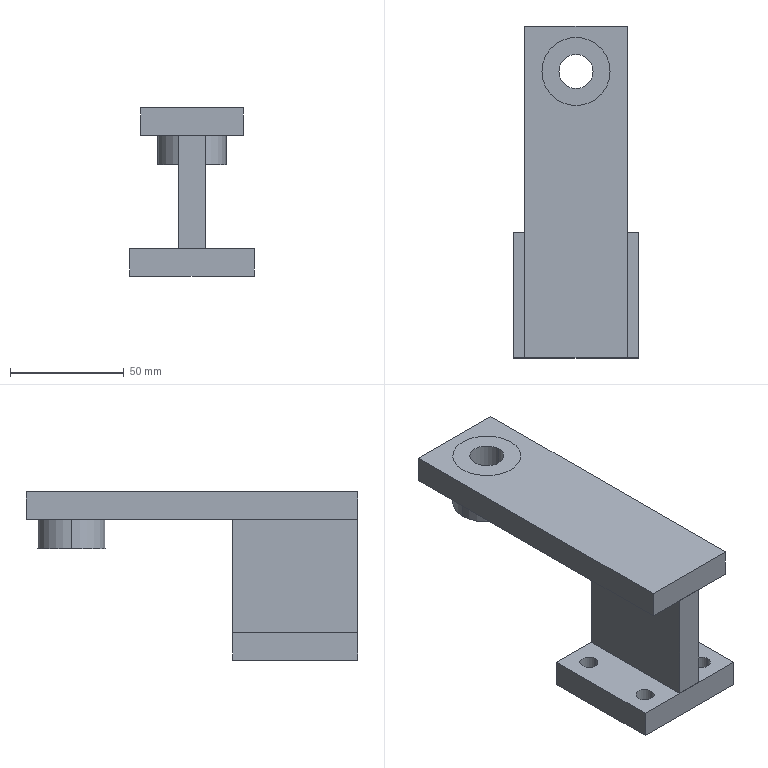Part | STEP file | Cuon T phu H01_14 | 4 solids | 34 faces | box 55 x 146 x 74 mm | volume 150499 mm3 | plane 20 | cylinder 14 | commonest cylinder face diameters 8 x8 30 x4 15 x2